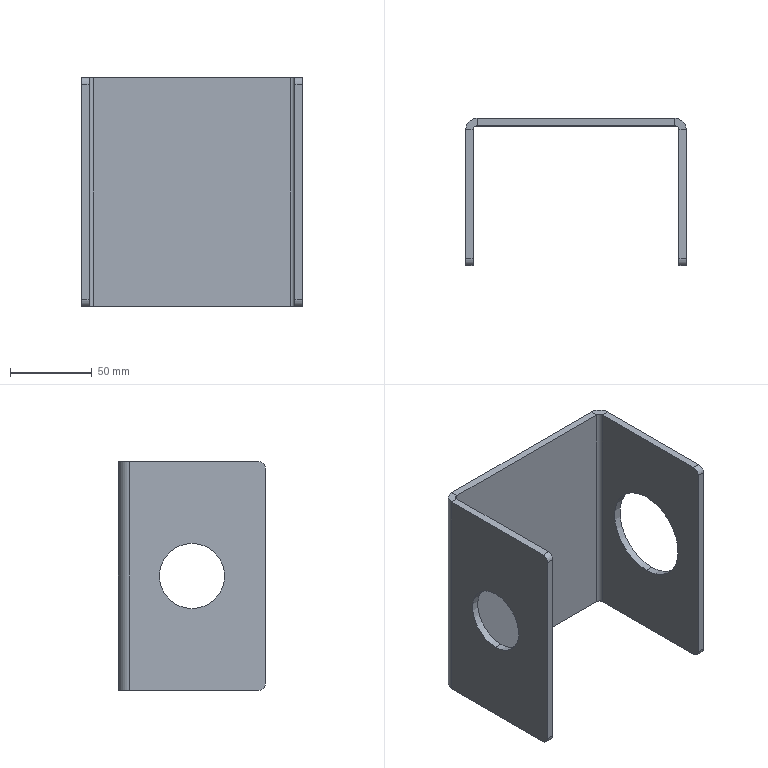Part | SolidWorks | features Cut 2, Fillet 1, FlatPattern 1, SMBaseFlange 1, SheetMetal 1, UnFold 1 | 1 solid | 30 faces | box 135 x 90 x 140 mm | volume 173803 mm3 | plane 18 | cylinder 12 | commonest cylinder face diameters 8 x4 5 x2 14 x2 40 x2 55 x2
STEP:
#1=CARTESIAN_POINT('',(63.,-45.,27.5));
#2=VERTEX_POINT('',#1);
#3=CARTESIAN_POINT('',(63.,-45.,-27.5));
#4=VERTEX_POINT('',#3);
#5=CARTESIAN_POINT('',(63.,-45.,0.));
#6=DIRECTION('',(1.,0.,0.));
#7=DIRECTION('',(0.,0.,-1.));
#8=AXIS2_PLACEMENT_3D('',#5,#6,#7);
#9=CIRCLE('',#8,27.5);
#10=EDGE_CURVE('',#2,#4,#9,.T.);
#11=ORIENTED_EDGE('',*,*,#10,.F.);
#12=CARTESIAN_POINT('',(67.5,-45.,27.5));
#13=VERTEX_POINT('',#12);
#14=CARTESIAN_POINT('',(57.5,-45.,27.5));
#15=DIRECTION('',(1.,0.,0.));
#16=VECTOR('',#15,1000.);
#17=LINE('',#14,#16);
#18=EDGE_CURVE('',#2,#13,#17,.T.);
#19=ORIENTED_EDGE('',*,*,#18,.T.);
#20=CARTESIAN_POINT('',(67.5,-45.,-27.5));
#21=VERTEX_POINT('',#20);
#22=CARTESIAN_POINT('',(67.5,-45.,0.));
#23=DIRECTION('',(1.,0.,0.));
#24=DIRECTION('',(0.,0.,-1.));
#25=AXIS2_PLACEMENT_3D('',#22,#23,#24);
#26=CIRCLE('',#25,27.5);
#27=EDGE_CURVE('',#13,#21,#26,.T.);
#28=ORIENTED_EDGE('',*,*,#27,.T.);
#29=CARTESIAN_POINT('',(57.5,-45.,-27.5));
#30=DIRECTION('',(1.,0.,0.));
#31=VECTOR('',#30,1000.);
#32=LINE('',#29,#31);
#33=EDGE_CURVE('',#4,#21,#32,.T.);
#34=ORIENTED_EDGE('',*,*,#33,.F.);
#35=EDGE_LOOP('',(#11,#19,#28,#34));
#36=FACE_OUTER_BOUND('',#35,.T.);
#37=CARTESIAN_POINT('',(57.5,-45.,0.));
#38=DIRECTION('',(1.,0.,0.));
#39=DIRECTION('',(0.,0.,-1.));
#40=AXIS2_PLACEMENT_3D('',#37,#38,#39);
#41=CYLINDRICAL_SURFACE('',#40,27.5);
#42=ADVANCED_FACE('',(#36),#41,.F.);
#43=CARTESIAN_POINT('',(-63.,-45.,-20.));
#44=VERTEX_POINT('',#43);
#45=CARTESIAN_POINT('',(-63.,-45.,20.));
#46=VERTEX_POINT('',#45);
#47=CARTESIAN_POINT('',(-63.,-45.,0.));
#48=DIRECTION('',(-1.,0.,0.));
#49=DIRECTION('',(0.,0.,1.));
#50=AXIS2_PLACEMENT_3D('',#47,#48,#49);
#51=CIRCLE('',#50,20.);
#52=EDGE_CURVE('',#44,#46,#51,.T.);
#53=ORIENTED_EDGE('',*,*,#52,.F.);
#54=CARTESIAN_POINT('',(-67.5,-45.,-20.));
#55=VERTEX_POINT('',#54);
#56=CARTESIAN_POINT('',(-57.5,-45.,-20.));
#57=DIRECTION('',(-1.,0.,0.));
#58=VECTOR('',#57,1000.);
#59=LINE('',#56,#58);
#60=EDGE_CURVE('',#44,#55,#59,.T.);
#61=ORIENTED_EDGE('',*,*,#60,.T.);
#62=CARTESIAN_POINT('',(-67.5,-45.,20.));
#63=VERTEX_POINT('',#62);
#64=CARTESIAN_POINT('',(-67.5,-45.,0.));
#65=DIRECTION('',(-1.,0.,0.));
#66=DIRECTION('',(0.,0.,1.));
#67=AXIS2_PLACEMENT_3D('',#64,#65,#66);
#68=CIRCLE('',#67,20.);
#69=EDGE_CURVE('',#55,#63,#68,.T.);
#70=ORIENTED_EDGE('',*,*,#69,.T.);
#71=CARTESIAN_POINT('',(-57.5,-45.,20.));
#72=DIRECTION('',(-1.,0.,0.));
#73=VECTOR('',#72,1000.);
#74=LINE('',#71,#73);
#75=EDGE_CURVE('',#46,#63,#74,.T.);
#76=ORIENTED_EDGE('',*,*,#75,.F.);
#77=EDGE_LOOP('',(#53,#61,#70,#76));
#78=FACE_OUTER_BOUND('',#77,.T.);
#79=CARTESIAN_POINT('',(-57.5,-45.,0.));
#80=DIRECTION('',(-1.,0.,0.));
#81=DIRECTION('',(0.,0.,1.));
#82=AXIS2_PLACEMENT_3D('',#79,#80,#81);
#83=CYLINDRICAL_SURFACE('',#82,20.);
#84=ADVANCED_FACE('',(#78),#83,.F.);
#85=CARTESIAN_POINT('',(-60.5,0.,70.));
#86=VERTEX_POINT('',#85);
#87=CARTESIAN_POINT('',(-60.5,-4.5,70.));
#88=VERTEX_POINT('',#87);
#89=CARTESIAN_POINT('',(-60.5,0.,70.));
#90=DIRECTION('',(0.,-1.,0.));
#91=VECTOR('',#90,1000.);
#92=LINE('',#89,#91);
#93=EDGE_CURVE('',#86,#88,#92,.T.);
#94=ORIENTED_EDGE('',*,*,#93,.F.);
#95=CARTESIAN_POINT('',(-67.5,-7.,70.));
#96=VERTEX_POINT('',#95);
#97=CARTESIAN_POINT('',(-60.5,-7.,70.));
#98=DIRECTION('',(0.,0.,-1.));
#99=DIRECTION('',(1.,0.,0.));
#100=AXIS2_PLACEMENT_3D('',#97,#98,#99);
#101=CIRCLE('',#100,7.);
#102=EDGE_CURVE('',#96,#86,#101,.T.);
#103=ORIENTED_EDGE('',*,*,#102,.F.);
#104=CARTESIAN_POINT('',(-63.,-7.,70.));
#105=VERTEX_POINT('',#104);
#106=CARTESIAN_POINT('',(-63.,-7.,70.));
#107=DIRECTION('',(-1.,0.,0.));
#108=VECTOR('',#107,1000.);
#109=LINE('',#106,#108);
#110=EDGE_CURVE('',#105,#96,#109,.T.);
#111=ORIENTED_EDGE('',*,*,#110,.F.);
#112=CARTESIAN_POINT('',(-60.5,-7.,70.));
#113=DIRECTION('',(0.,0.,-1.));
#114=DIRECTION('',(1.,0.,0.));
#115=AXIS2_PLACEMENT_3D('',#112,#113,#114);
#116=CIRCLE('',#115,2.5);
#117=EDGE_CURVE('',#105,#88,#116,.T.);
#118=ORIENTED_EDGE('',*,*,#117,.T.);
#119=EDGE_LOOP('',(#94,#103,#111,#118));
#120=FACE_OUTER_BOUND('',#119,.T.);
#121=CARTESIAN_POINT('',(-60.5,0.,70.));
#122=DIRECTION('',(0.,0.,1.));
#123=DIRECTION('',(1.,0.,0.));
#124=AXIS2_PLACEMENT_3D('',#121,#122,#123);
#125=PLANE('',#124);
#126=ADVANCED_FACE('',(#120),#125,.T.);
#127=CARTESIAN_POINT('',(60.5,0.,70.));
#128=VERTEX_POINT('',#127);
#129=CARTESIAN_POINT('',(-67.5,0.,70.));
#130=DIRECTION('',(1.,0.,0.));
#131=VECTOR('',#130,1000.);
#132=LINE('',#129,#131);
#133=EDGE_CURVE('',#86,#128,#132,.T.);
#134=ORIENTED_EDGE('',*,*,#133,.F.);
#135=ORIENTED_EDGE('',*,*,#93,.T.);
#136=CARTESIAN_POINT('',(60.5,-4.5,70.));
#137=VERTEX_POINT('',#136);
#138=CARTESIAN_POINT('',(-67.5,-4.5,70.));
#139=DIRECTION('',(1.,0.,0.));
#140=VECTOR('',#139,1000.);
#141=LINE('',#138,#140);
#142=EDGE_CURVE('',#88,#137,#141,.T.);
#143=ORIENTED_EDGE('',*,*,#142,.T.);
#144=CARTESIAN_POINT('',(60.5,-4.5,70.));
#145=DIRECTION('',(0.,1.,0.));
#146=VECTOR('',#145,1000.);
#147=LINE('',#144,#146);
#148=EDGE_CURVE('',#137,#128,#147,.T.);
#149=ORIENTED_EDGE('',*,*,#148,.T.);
#150=EDGE_LOOP('',(#134,#135,#143,#149));
#151=FACE_OUTER_BOUND('',#150,.T.);
#152=CARTESIAN_POINT('',(-63.,-7.,70.));
#153=DIRECTION('',(0.,0.,1.));
#154=DIRECTION('',(1.,0.,0.));
#155=AXIS2_PLACEMENT_3D('',#152,#153,#154);
#156=PLANE('',#155);
#157=ADVANCED_FACE('',(#151),#156,.T.);
#158=CARTESIAN_POINT('',(-67.5,-7.,-70.));
#159=VERTEX_POINT('',#158);
#160=CARTESIAN_POINT('',(-63.,-7.,-70.));
#161=VERTEX_POINT('',#160);
#162=CARTESIAN_POINT('',(-67.5,-7.,-70.));
#163=DIRECTION('',(1.,0.,0.));
#164=VECTOR('',#163,1000.);
#165=LINE('',#162,#164);
#166=EDGE_CURVE('',#159,#161,#165,.T.);
#167=ORIENTED_EDGE('',*,*,#166,.F.);
#168=CARTESIAN_POINT('',(-60.5,0.,-70.));
#169=VERTEX_POINT('',#168);
#170=CARTESIAN_POINT('',(-60.5,-7.,-70.));
#171=DIRECTION('',(0.,0.,-1.));
#172=DIRECTION('',(1.,0.,0.));
#173=AXIS2_PLACEMENT_3D('',#170,#171,#172);
#174=CIRCLE('',#173,7.);
#175=EDGE_CURVE('',#159,#169,#174,.T.);
#176=ORIENTED_EDGE('',*,*,#175,.T.);
#177=CARTESIAN_POINT('',(-60.5,-4.5,-70.));
#178=VERTEX_POINT('',#177);
#179=CARTESIAN_POINT('',(-60.5,-4.5,-70.));
#180=DIRECTION('',(0.,1.,0.));
#181=VECTOR('',#180,1000.);
#182=LINE('',#179,#181);
#183=EDGE_CURVE('',#178,#169,#182,.T.);
#184=ORIENTED_EDGE('',*,*,#183,.F.);
#185=CARTESIAN_POINT('',(-60.5,-7.,-70.));
#186=DIRECTION('',(0.,0.,-1.));
#187=DIRECTION('',(1.,0.,0.));
#188=AXIS2_PLACEMENT_3D('',#185,#186,#187);
#189=CIRCLE('',#188,2.5);
#190=EDGE_CURVE('',#161,#178,#189,.T.);
#191=ORIENTED_EDGE('',*,*,#190,.F.);
#192=EDGE_LOOP('',(#167,#176,#184,#191));
#193=FACE_OUTER_BOUND('',#192,.T.);
#194=CARTESIAN_POINT('',(-67.5,-7.,-70.));
#195=DIRECTION('',(0.,0.,-1.));
#196=DIRECTION('',(-1.,0.,0.));
#197=AXIS2_PLACEMENT_3D('',#194,#195,#196);
#198=PLANE('',#197);
#199=ADVANCED_FACE('',(#193),#198,.T.);
#200=CARTESIAN_POINT('',(-63.,-86.,-70.));
#201=VERTEX_POINT('',#200);
#202=CARTESIAN_POINT('',(-63.,-90.,-70.));
#203=DIRECTION('',(0.,1.,0.));
#204=VECTOR('',#203,1000.);
#205=LINE('',#202,#204);
#206=EDGE_CURVE('',#201,#161,#205,.T.);
#207=ORIENTED_EDGE('',*,*,#206,.F.);
#208=CARTESIAN_POINT('',(-67.5,-86.,-70.));
#209=VERTEX_POINT('',#208);
#210=CARTESIAN_POINT('',(-60.5,-86.,-70.));
#211=DIRECTION('',(-1.,0.,0.));
#212=VECTOR('',#211,1000.);
#213=LINE('',#210,#212);
#214=EDGE_CURVE('',#201,#209,#213,.T.);
#215=ORIENTED_EDGE('',*,*,#214,.T.);
#216=CARTESIAN_POINT('',(-67.5,-90.,-70.));
#217=DIRECTION('',(0.,1.,0.));
#218=VECTOR('',#217,1000.);
#219=LINE('',#216,#218);
#220=EDGE_CURVE('',#209,#159,#219,.T.);
#221=ORIENTED_EDGE('',*,*,#220,.T.);
#222=ORIENTED_EDGE('',*,*,#166,.T.);
#223=EDGE_LOOP('',(#207,#215,#221,#222));
#224=FACE_OUTER_BOUND('',#223,.T.);
#225=CARTESIAN_POINT('',(-60.5,-4.5,-70.));
#226=DIRECTION('',(0.,0.,-1.));
#227=DIRECTION('',(-1.,0.,0.));
#228=AXIS2_PLACEMENT_3D('',#225,#226,#227);
#229=PLANE('',#228);
#230=ADVANCED_FACE('',(#224),#229,.T.);
#231=CARTESIAN_POINT('',(67.5,-7.,70.));
#232=VERTEX_POINT('',#231);
#233=CARTESIAN_POINT('',(63.,-7.,70.));
#234=VERTEX_POINT('',#233);
#235=CARTESIAN_POINT('',(67.5,-7.,70.));
#236=DIRECTION('',(-1.,0.,0.));
#237=VECTOR('',#236,1000.);
#238=LINE('',#235,#237);
#239=EDGE_CURVE('',#232,#234,#238,.T.);
#240=ORIENTED_EDGE('',*,*,#239,.F.);
#241=CARTESIAN_POINT('',(60.5,-7.,70.));
#242=DIRECTION('',(0.,0.,-1.));
#243=DIRECTION('',(1.,0.,0.));
#244=AXIS2_PLACEMENT_3D('',#241,#242,#243);
#245=CIRCLE('',#244,7.);
#246=EDGE_CURVE('',#128,#232,#245,.T.);
#247=ORIENTED_EDGE('',*,*,#246,.F.);
#248=ORIENTED_EDGE('',*,*,#148,.F.);
#249=CARTESIAN_POINT('',(60.5,-7.,70.));
#250=DIRECTION('',(0.,0.,-1.));
#251=DIRECTION('',(1.,0.,0.));
#252=AXIS2_PLACEMENT_3D('',#249,#250,#251);
#253=CIRCLE('',#252,2.5);
#254=EDGE_CURVE('',#137,#234,#253,.T.);
#255=ORIENTED_EDGE('',*,*,#254,.T.);
#256=EDGE_LOOP('',(#240,#247,#248,#255));
#257=FACE_OUTER_BOUND('',#256,.T.);
#258=CARTESIAN_POINT('',(67.5,-7.,70.));
#259=DIRECTION('',(0.,0.,1.));
#260=DIRECTION('',(1.,0.,0.));
#261=AXIS2_PLACEMENT_3D('',#258,#259,#260);
#262=PLANE('',#261);
#263=ADVANCED_FACE('',(#257),#262,.T.);
#264=CARTESIAN_POINT('',(63.,-86.,70.));
#265=VERTEX_POINT('',#264);
#266=CARTESIAN_POINT('',(63.,0.,70.));
#267=DIRECTION('',(0.,-1.,0.));
#268=VECTOR('',#267,1000.);
#269=LINE('',#266,#268);
#270=EDGE_CURVE('',#234,#265,#269,.T.);
#271=ORIENTED_EDGE('',*,*,#270,.T.);
#272=CARTESIAN_POINT('',(67.5,-86.,70.));
#273=VERTEX_POINT('',#272);
#274=CARTESIAN_POINT('',(60.5,-86.,70.));
#275=DIRECTION('',(1.,0.,0.));
#276=VECTOR('',#275,1000.);
#277=LINE('',#274,#276);
#278=EDGE_CURVE('',#265,#273,#277,.T.);
#279=ORIENTED_EDGE('',*,*,#278,.T.);
#280=CARTESIAN_POINT('',(67.5,0.,70.));
#281=DIRECTION('',(0.,-1.,0.));
#282=VECTOR('',#281,1000.);
#283=LINE('',#280,#282);
#284=EDGE_CURVE('',#232,#273,#283,.T.);
#285=ORIENTED_EDGE('',*,*,#284,.F.);
#286=ORIENTED_EDGE('',*,*,#239,.T.);
#287=EDGE_LOOP('',(#271,#279,#285,#286));
#288=FACE_OUTER_BOUND('',#287,.T.);
#289=CARTESIAN_POINT('',(60.5,-4.5,70.));
#290=DIRECTION('',(0.,0.,1.));
#291=DIRECTION('',(1.,0.,0.));
#292=AXIS2_PLACEMENT_3D('',#289,#290,#291);
#293=PLANE('',#292);
#294=ADVANCED_FACE('',(#288),#293,.T.);
#295=CARTESIAN_POINT('',(60.5,0.,-70.));
#296=VERTEX_POINT('',#295);
#297=CARTESIAN_POINT('',(60.5,-4.5,-70.));
#298=VERTEX_POINT('',#297);
#299=CARTESIAN_POINT('',(60.5,0.,-70.));
#300=DIRECTION('',(0.,-1.,0.));
#301=VECTOR('',#300,1000.);
#302=LINE('',#299,#301);
#303=EDGE_CURVE('',#296,#298,#302,.T.);
#304=ORIENTED_EDGE('',*,*,#303,.F.);
#305=CARTESIAN_POINT('',(67.5,-7.,-70.));
#306=VERTEX_POINT('',#305);
#307=CARTESIAN_POINT('',(60.5,-7.,-70.));
#308=DIRECTION('',(0.,0.,-1.));
#309=DIRECTION('',(1.,0.,0.));
#310=AXIS2_PLACEMENT_3D('',#307,#308,#309);
#311=CIRCLE('',#310,7.);
#312=EDGE_CURVE('',#296,#306,#311,.T.);
#313=ORIENTED_EDGE('',*,*,#312,.T.);
#314=CARTESIAN_POINT('',(63.,-7.,-70.));
#315=VERTEX_POINT('',#314);
#316=CARTESIAN_POINT('',(63.,-7.,-70.));
#317=DIRECTION('',(1.,0.,0.));
#318=VECTOR('',#317,1000.);
#319=LINE('',#316,#318);
#320=EDGE_CURVE('',#315,#306,#319,.T.);
#321=ORIENTED_EDGE('',*,*,#320,.F.);
#322=CARTESIAN_POINT('',(60.5,-7.,-70.));
#323=DIRECTION('',(0.,0.,-1.));
#324=DIRECTION('',(1.,0.,0.));
#325=AXIS2_PLACEMENT_3D('',#322,#323,#324);
#326=CIRCLE('',#325,2.5);
#327=EDGE_CURVE('',#298,#315,#326,.T.);
#328=ORIENTED_EDGE('',*,*,#327,.F.);
#329=EDGE_LOOP('',(#304,#313,#321,#328));
#330=FACE_OUTER_BOUND('',#329,.T.);
#331=CARTESIAN_POINT('',(60.5,0.,-70.));
#332=DIRECTION('',(0.,0.,-1.));
#333=DIRECTION('',(-1.,0.,0.));
#334=AXIS2_PLACEMENT_3D('',#331,#332,#333);
#335=PLANE('',#334);
#336=ADVANCED_FACE('',(#330),#335,.T.);
#337=CARTESIAN_POINT('',(-67.5,0.,-70.));
#338=DIRECTION('',(1.,0.,0.));
#339=VECTOR('',#338,1000.);
#340=LINE('',#337,#339);
#341=EDGE_CURVE('',#169,#296,#340,.T.);
#342=ORIENTED_EDGE('',*,*,#341,.T.);
#343=ORIENTED_EDGE('',*,*,#303,.T.);
#344=CARTESIAN_POINT('',(-67.5,-4.5,-70.));
#345=DIRECTION('',(1.,0.,0.));
#346=VECTOR('',#345,1000.);
#347=LINE('',#344,#346);
#348=EDGE_CURVE('',#178,#298,#347,.T.);
#349=ORIENTED_EDGE('',*,*,#348,.F.);
#350=ORIENTED_EDGE('',*,*,#183,.T.);
#351=EDGE_LOOP('',(#342,#343,#349,#350));
#352=FACE_OUTER_BOUND('',#351,.T.);
#353=CARTESIAN_POINT('',(63.,-7.,-70.));
#354=DIRECTION('',(0.,0.,-1.));
#355=DIRECTION('',(-1.,0.,0.));
#356=AXIS2_PLACEMENT_3D('',#353,#354,#355);
#357=PLANE('',#356);
#358=ADVANCED_FACE('',(#352),#357,.T.);
#359=CARTESIAN_POINT('',(63.,-45.,0.));
#360=DIRECTION('',(1.,0.,0.));
#361=DIRECTION('',(0.,0.,-1.));
#362=AXIS2_PLACEMENT_3D('',#359,#360,#361);
#363=CIRCLE('',#362,27.5);
#364=EDGE_CURVE('',#4,#2,#363,.T.);
#365=ORIENTED_EDGE('',*,*,#364,.T.);
#366=ORIENTED_EDGE('',*,*,#10,.T.);
#367=EDGE_LOOP('',(#365,#366));
#368=FACE_BOUND('',#367,.T.);
#369=CARTESIAN_POINT('',(63.,-86.,-70.));
#370=VERTEX_POINT('',#369);
#371=CARTESIAN_POINT('',(63.,0.,-70.));
#372=DIRECTION('',(0.,-1.,0.));
#373=VECTOR('',#372,1000.);
#374=LINE('',#371,#373);
#375=EDGE_CURVE('',#315,#370,#374,.T.);
#376=ORIENTED_EDGE('',*,*,#375,.T.);
#377=CARTESIAN_POINT('',(63.,-90.,-66.));
#378=VERTEX_POINT('',#377);
#379=CARTESIAN_POINT('',(63.,-86.,-66.));
#380=DIRECTION('',(-1.,0.,0.));
#381=DIRECTION('',(0.,0.,-1.));
#382=AXIS2_PLACEMENT_3D('',#379,#380,#381);
#383=CIRCLE('',#382,4.);
#384=EDGE_CURVE('',#370,#378,#383,.T.);
#385=ORIENTED_EDGE('',*,*,#384,.T.);
#386=CARTESIAN_POINT('',(63.,-90.,66.));
#387=VERTEX_POINT('',#386);
#388=CARTESIAN_POINT('',(63.,-90.,70.));
#389=DIRECTION('',(0.,0.,-1.));
#390=VECTOR('',#389,1000.);
#391=LINE('',#388,#390);
#392=EDGE_CURVE('',#387,#378,#391,.T.);
#393=ORIENTED_EDGE('',*,*,#392,.F.);
#394=CARTESIAN_POINT('',(63.,-86.,66.));
#395=DIRECTION('',(-1.,0.,0.));
#396=DIRECTION('',(0.,0.,-1.));
#397=AXIS2_PLACEMENT_3D('',#394,#395,#396);
#398=CIRCLE('',#397,4.);
#399=EDGE_CURVE('',#387,#265,#398,.T.);
#400=ORIENTED_EDGE('',*,*,#399,.T.);
#401=ORIENTED_EDGE('',*,*,#270,.F.);
#402=CARTESIAN_POINT('',(63.,-7.,70.));
#403=DIRECTION('',(0.,0.,-1.));
#404=VECTOR('',#403,1000.);
#405=LINE('',#402,#404);
#406=EDGE_CURVE('',#234,#315,#405,.T.);
#407=ORIENTED_EDGE('',*,*,#406,.T.);
#408=EDGE_LOOP('',(#376,#385,#393,#400,#401,#407));
#409=FACE_OUTER_BOUND('',#408,.T.);
#410=CARTESIAN_POINT('',(63.,0.,70.));
#411=DIRECTION('',(1.,0.,0.));
#412=DIRECTION('',(0.,0.,-1.));
#413=AXIS2_PLACEMENT_3D('',#410,#411,#412);
#414=PLANE('',#413);
#415=ADVANCED_FACE('',(#368,#409),#414,.F.);
#416=ORIENTED_EDGE('',*,*,#392,.T.);
#417=CARTESIAN_POINT('',(67.5,-90.,-66.));
#418=VERTEX_POINT('',#417);
#419=CARTESIAN_POINT('',(67.5,-90.,-66.));
#420=DIRECTION('',(1.,0.,0.));
#421=VECTOR('',#420,1000.);
#422=LINE('',#419,#421);
#423=EDGE_CURVE('',#378,#418,#422,.T.);
#424=ORIENTED_EDGE('',*,*,#423,.T.);
#425=CARTESIAN_POINT('',(67.5,-90.,66.));
#426=VERTEX_POINT('',#425);
#427=CARTESIAN_POINT('',(67.5,-90.,70.));
#428=DIRECTION('',(0.,0.,-1.));
#429=VECTOR('',#428,1000.);
#430=LINE('',#427,#429);
#431=EDGE_CURVE('',#426,#418,#430,.T.);
#432=ORIENTED_EDGE('',*,*,#431,.F.);
#433=CARTESIAN_POINT('',(67.5,-90.,66.));
#434=DIRECTION('',(-1.,0.,0.));
#435=VECTOR('',#434,1000.);
#436=LINE('',#433,#435);
#437=EDGE_CURVE('',#426,#387,#436,.T.);
#438=ORIENTED_EDGE('',*,*,#437,.T.);
#439=EDGE_LOOP('',(#416,#424,#432,#438));
#440=FACE_OUTER_BOUND('',#439,.T.);
#441=CARTESIAN_POINT('',(67.5,-90.,70.));
#442=DIRECTION('',(0.,-1.,0.));
#443=DIRECTION('',(0.,0.,-1.));
#444=AXIS2_PLACEMENT_3D('',#441,#442,#443);
#445=PLANE('',#444);
#446=ADVANCED_FACE('',(#440),#445,.T.);
#447=CARTESIAN_POINT('',(67.5,-45.,0.));
#448=DIRECTION('',(1.,0.,0.));
#449=DIRECTION('',(0.,0.,-1.));
#450=AXIS2_PLACEMENT_3D('',#447,#448,#449);
#451=CIRCLE('',#450,27.5);
#452=EDGE_CURVE('',#21,#13,#451,.T.);
#453=ORIENTED_EDGE('',*,*,#452,.F.);
#454=ORIENTED_EDGE('',*,*,#27,.F.);
#455=EDGE_LOOP('',(#453,#454));
#456=FACE_BOUND('',#455,.T.);
#457=ORIENTED_EDGE('',*,*,#431,.T.);
#458=CARTESIAN_POINT('',(67.5,-86.,-70.));
#459=VERTEX_POINT('',#458);
#460=CARTESIAN_POINT('',(67.5,-86.,-66.));
#461=DIRECTION('',(1.,0.,0.));
#462=DIRECTION('',(0.,0.,-1.));
#463=AXIS2_PLACEMENT_3D('',#460,#461,#462);
#464=CIRCLE('',#463,4.);
#465=EDGE_CURVE('',#418,#459,#464,.T.);
#466=ORIENTED_EDGE('',*,*,#465,.T.);
#467=CARTESIAN_POINT('',(67.5,0.,-70.));
#468=DIRECTION('',(0.,-1.,0.));
#469=VECTOR('',#468,1000.);
#470=LINE('',#467,#469);
#471=EDGE_CURVE('',#306,#459,#470,.T.);
#472=ORIENTED_EDGE('',*,*,#471,.F.);
#473=CARTESIAN_POINT('',(67.5,-7.,70.));
#474=DIRECTION('',(0.,0.,-1.));
#475=VECTOR('',#474,1000.);
#476=LINE('',#473,#475);
#477=EDGE_CURVE('',#232,#306,#476,.T.);
#478=ORIENTED_EDGE('',*,*,#477,.F.);
#479=ORIENTED_EDGE('',*,*,#284,.T.);
#480=CARTESIAN_POINT('',(67.5,-86.,66.));
#481=DIRECTION('',(1.,0.,0.));
#482=DIRECTION('',(0.,0.,-1.));
#483=AXIS2_PLACEMENT_3D('',#480,#481,#482);
#484=CIRCLE('',#483,4.);
#485=EDGE_CURVE('',#273,#426,#484,.T.);
#486=ORIENTED_EDGE('',*,*,#485,.T.);
#487=EDGE_LOOP('',(#457,#466,#472,#478,#479,#486));
#488=FACE_OUTER_BOUND('',#487,.T.);
#489=CARTESIAN_POINT('',(67.5,0.,70.));
#490=DIRECTION('',(1.,0.,0.));
#491=DIRECTION('',(0.,0.,-1.));
#492=AXIS2_PLACEMENT_3D('',#489,#490,#491);
#493=PLANE('',#492);
#494=ADVANCED_FACE('',(#456,#488),#493,.T.);
#495=ORIENTED_EDGE('',*,*,#312,.F.);
#496=CARTESIAN_POINT('',(60.5,0.,70.));
#497=DIRECTION('',(0.,0.,-1.));
#498=VECTOR('',#497,1000.);
#499=LINE('',#496,#498);
#500=EDGE_CURVE('',#128,#296,#499,.T.);
#501=ORIENTED_EDGE('',*,*,#500,.F.);
#502=ORIENTED_EDGE('',*,*,#246,.T.);
#503=ORIENTED_EDGE('',*,*,#477,.T.);
#504=EDGE_LOOP('',(#495,#501,#502,#503));
#505=FACE_OUTER_BOUND('',#504,.T.);
#506=CARTESIAN_POINT('',(60.5,-7.,70.));
#507=DIRECTION('',(0.,0.,-1.));
#508=DIRECTION('',(-1.,0.,0.));
#509=AXIS2_PLACEMENT_3D('',#506,#507,#508);
#510=CYLINDRICAL_SURFACE('',#509,7.);
#511=ADVANCED_FACE('',(#505),#510,.T.);
#512=ORIENTED_EDGE('',*,*,#341,.F.);
#513=CARTESIAN_POINT('',(-60.5,0.,70.));
#514=DIRECTION('',(0.,0.,-1.));
#515=VECTOR('',#514,1000.);
#516=LINE('',#513,#515);
#517=EDGE_CURVE('',#86,#169,#516,.T.);
#518=ORIENTED_EDGE('',*,*,#517,.F.);
#519=ORIENTED_EDGE('',*,*,#133,.T.);
#520=ORIENTED_EDGE('',*,*,#500,.T.);
#521=EDGE_LOOP('',(#512,#518,#519,#520));
#522=FACE_OUTER_BOUND('',#521,.T.);
#523=CARTESIAN_POINT('',(-67.5,0.,70.));
#524=DIRECTION('',(0.,1.,0.));
#525=DIRECTION('',(0.,0.,1.));
#526=AXIS2_PLACEMENT_3D('',#523,#524,#525);
#527=PLANE('',#526);
#528=ADVANCED_FACE('',(#522),#527,.T.);
#529=ORIENTED_EDGE('',*,*,#175,.F.);
#530=CARTESIAN_POINT('',(-67.5,-7.,70.));
#531=DIRECTION('',(0.,0.,-1.));
#532=VECTOR('',#531,1000.);
#533=LINE('',#530,#532);
#534=EDGE_CURVE('',#96,#159,#533,.T.);
#535=ORIENTED_EDGE('',*,*,#534,.F.);
#536=ORIENTED_EDGE('',*,*,#102,.T.);
#537=ORIENTED_EDGE('',*,*,#517,.T.);
#538=EDGE_LOOP('',(#529,#535,#536,#537));
#539=FACE_OUTER_BOUND('',#538,.T.);
#540=CARTESIAN_POINT('',(-60.5,-7.,70.));
#541=DIRECTION('',(0.,0.,-1.));
#542=DIRECTION('',(-1.,0.,0.));
#543=AXIS2_PLACEMENT_3D('',#540,#541,#542);
#544=CYLINDRICAL_SURFACE('',#543,7.);
#545=ADVANCED_FACE('',(#539),#544,.T.);
#546=CARTESIAN_POINT('',(-67.5,-45.,0.));
#547=DIRECTION('',(-1.,0.,0.));
#548=DIRECTION('',(0.,0.,1.));
#549=AXIS2_PLACEMENT_3D('',#546,#547,#548);
#550=CIRCLE('',#549,20.);
#551=EDGE_CURVE('',#63,#55,#550,.T.);
#552=ORIENTED_EDGE('',*,*,#551,.F.);
#553=ORIENTED_EDGE('',*,*,#69,.F.);
#554=EDGE_LOOP('',(#552,#553));
#555=FACE_BOUND('',#554,.T.);
#556=ORIENTED_EDGE('',*,*,#220,.F.);
#557=CARTESIAN_POINT('',(-67.5,-90.,-66.));
#558=VERTEX_POINT('',#557);
#559=CARTESIAN_POINT('',(-67.5,-86.,-66.));
#560=DIRECTION('',(-1.,0.,0.));
#561=DIRECTION('',(0.,0.,1.));
#562=AXIS2_PLACEMENT_3D('',#559,#560,#561);
#563=CIRCLE('',#562,4.);
#564=EDGE_CURVE('',#209,#558,#563,.T.);
#565=ORIENTED_EDGE('',*,*,#564,.T.);
#566=CARTESIAN_POINT('',(-67.5,-90.,66.));
#567=VERTEX_POINT('',#566);
#568=CARTESIAN_POINT('',(-67.5,-90.,70.));
#569=DIRECTION('',(0.,0.,-1.));
#570=VECTOR('',#569,1000.);
#571=LINE('',#568,#570);
#572=EDGE_CURVE('',#567,#558,#571,.T.);
#573=ORIENTED_EDGE('',*,*,#572,.F.);
#574=CARTESIAN_POINT('',(-67.5,-86.,70.));
#575=VERTEX_POINT('',#574);
#576=CARTESIAN_POINT('',(-67.5,-86.,66.));
#577=DIRECTION('',(-1.,0.,0.));
#578=DIRECTION('',(0.,0.,1.));
#579=AXIS2_PLACEMENT_3D('',#576,#577,#578);
#580=CIRCLE('',#579,4.);
#581=EDGE_CURVE('',#567,#575,#580,.T.);
#582=ORIENTED_EDGE('',*,*,#581,.T.);
#583=CARTESIAN_POINT('',(-67.5,-90.,70.));
#584=DIRECTION('',(0.,1.,0.));
#585=VECTOR('',#584,1000.);
#586=LINE('',#583,#585);
#587=EDGE_CURVE('',#575,#96,#586,.T.);
#588=ORIENTED_EDGE('',*,*,#587,.T.);
#589=ORIENTED_EDGE('',*,*,#534,.T.);
#590=EDGE_LOOP('',(#556,#565,#573,#582,#588,#589));
#591=FACE_OUTER_BOUND('',#590,.T.);
#592=CARTESIAN_POINT('',(-67.5,-90.,70.));
#593=DIRECTION('',(-1.,0.,0.));
#594=DIRECTION('',(0.,0.,1.));
#595=AXIS2_PLACEMENT_3D('',#592,#593,#594);
#596=PLANE('',#595);
#597=ADVANCED_FACE('',(#555,#591),#596,.T.);
#598=ORIENTED_EDGE('',*,*,#572,.T.);
#599=CARTESIAN_POINT('',(-63.,-90.,-66.));
#600=VERTEX_POINT('',#599);
#601=CARTESIAN_POINT('',(-63.,-90.,-66.));
#602=DIRECTION('',(1.,0.,0.));
#603=VECTOR('',#602,1000.);
#604=LINE('',#601,#603);
#605=EDGE_CURVE('',#558,#600,#604,.T.);
#606=ORIENTED_EDGE('',*,*,#605,.T.);
#607=CARTESIAN_POINT('',(-63.,-90.,66.));
#608=VERTEX_POINT('',#607);
#609=CARTESIAN_POINT('',(-63.,-90.,70.));
#610=DIRECTION('',(0.,0.,-1.));
#611=VECTOR('',#610,1000.);
#612=LINE('',#609,#611);
#613=EDGE_CURVE('',#608,#600,#612,.T.);
#614=ORIENTED_EDGE('',*,*,#613,.F.);
#615=CARTESIAN_POINT('',(-63.,-90.,66.));
#616=DIRECTION('',(-1.,0.,0.));
#617=VECTOR('',#616,1000.);
#618=LINE('',#615,#617);
#619=EDGE_CURVE('',#608,#567,#618,.T.);
#620=ORIENTED_EDGE('',*,*,#619,.T.);
#621=EDGE_LOOP('',(#598,#606,#614,#620));
#622=FACE_OUTER_BOUND('',#621,.T.);
#623=CARTESIAN_POINT('',(-63.,-90.,70.));
#624=DIRECTION('',(0.,-1.,0.));
#625=DIRECTION('',(0.,0.,-1.));
#626=AXIS2_PLACEMENT_3D('',#623,#624,#625);
#627=PLANE('',#626);
#628=ADVANCED_FACE('',(#622),#627,.T.);
#629=CARTESIAN_POINT('',(-63.,-45.,0.));
#630=DIRECTION('',(-1.,0.,0.));
#631=DIRECTION('',(0.,0.,1.));
#632=AXIS2_PLACEMENT_3D('',#629,#630,#631);
#633=CIRCLE('',#632,20.);
#634=EDGE_CURVE('',#46,#44,#633,.T.);
#635=ORIENTED_EDGE('',*,*,#634,.T.);
#636=ORIENTED_EDGE('',*,*,#52,.T.);
#637=EDGE_LOOP('',(#635,#636));
#638=FACE_BOUND('',#637,.T.);
#639=ORIENTED_EDGE('',*,*,#613,.T.);
#640=CARTESIAN_POINT('',(-63.,-86.,-66.));
#641=DIRECTION('',(1.,0.,0.));
#642=DIRECTION('',(0.,0.,1.));
#643=AXIS2_PLACEMENT_3D('',#640,#641,#642);
#644=CIRCLE('',#643,4.);
#645=EDGE_CURVE('',#600,#201,#644,.T.);
#646=ORIENTED_EDGE('',*,*,#645,.T.);
#647=ORIENTED_EDGE('',*,*,#206,.T.);
#648=CARTESIAN_POINT('',(-63.,-7.,70.));
#649=DIRECTION('',(0.,0.,-1.));
#650=VECTOR('',#649,1000.);
#651=LINE('',#648,#650);
#652=EDGE_CURVE('',#105,#161,#651,.T.);
#653=ORIENTED_EDGE('',*,*,#652,.F.);
#654=CARTESIAN_POINT('',(-63.,-86.,70.));
#655=VERTEX_POINT('',#654);
#656=CARTESIAN_POINT('',(-63.,-90.,70.));
#657=DIRECTION('',(0.,1.,0.));
#658=VECTOR('',#657,1000.);
#659=LINE('',#656,#658);
#660=EDGE_CURVE('',#655,#105,#659,.T.);
#661=ORIENTED_EDGE('',*,*,#660,.F.);
#662=CARTESIAN_POINT('',(-63.,-86.,66.));
#663=DIRECTION('',(1.,0.,0.));
#664=DIRECTION('',(0.,0.,1.));
#665=AXIS2_PLACEMENT_3D('',#662,#663,#664);
#666=CIRCLE('',#665,4.);
#667=EDGE_CURVE('',#655,#608,#666,.T.);
#668=ORIENTED_EDGE('',*,*,#667,.T.);
#669=EDGE_LOOP('',(#639,#646,#647,#653,#661,#668));
#670=FACE_OUTER_BOUND('',#669,.T.);
#671=CARTESIAN_POINT('',(-63.,-90.,70.));
#672=DIRECTION('',(-1.,0.,0.));
#673=DIRECTION('',(0.,0.,1.));
#674=AXIS2_PLACEMENT_3D('',#671,#672,#673);
#675=PLANE('',#674);
#676=ADVANCED_FACE('',(#638,#670),#675,.F.);
#677=ORIENTED_EDGE('',*,*,#190,.T.);
#678=CARTESIAN_POINT('',(-60.5,-4.5,70.));
#679=DIRECTION('',(0.,0.,-1.));
#680=VECTOR('',#679,1000.);
#681=LINE('',#678,#680);
#682=EDGE_CURVE('',#88,#178,#681,.T.);
#683=ORIENTED_EDGE('',*,*,#682,.F.);
#684=ORIENTED_EDGE('',*,*,#117,.F.);
#685=ORIENTED_EDGE('',*,*,#652,.T.);
#686=EDGE_LOOP('',(#677,#683,#684,#685));
#687=FACE_OUTER_BOUND('',#686,.T.);
#688=CARTESIAN_POINT('',(-60.5,-7.,70.));
#689=DIRECTION('',(0.,0.,-1.));
#690=DIRECTION('',(-1.,0.,0.));
#691=AXIS2_PLACEMENT_3D('',#688,#689,#690);
#692=CYLINDRICAL_SURFACE('',#691,2.5);
#693=ADVANCED_FACE('',(#687),#692,.F.);
#694=ORIENTED_EDGE('',*,*,#348,.T.);
#695=CARTESIAN_POINT('',(60.5,-4.5,70.));
#696=DIRECTION('',(0.,0.,-1.));
#697=VECTOR('',#696,1000.);
#698=LINE('',#695,#697);
#699=EDGE_CURVE('',#137,#298,#698,.T.);
#700=ORIENTED_EDGE('',*,*,#699,.F.);
#701=ORIENTED_EDGE('',*,*,#142,.F.);
#702=ORIENTED_EDGE('',*,*,#682,.T.);
#703=EDGE_LOOP('',(#694,#700,#701,#702));
#704=FACE_OUTER_BOUND('',#703,.T.);
#705=CARTESIAN_POINT('',(-67.5,-4.5,70.));
#706=DIRECTION('',(0.,1.,0.));
#707=DIRECTION('',(0.,0.,1.));
#708=AXIS2_PLACEMENT_3D('',#705,#706,#707);
#709=PLANE('',#708);
#710=ADVANCED_FACE('',(#704),#709,.F.);
#711=ORIENTED_EDGE('',*,*,#327,.T.);
#712=ORIENTED_EDGE('',*,*,#406,.F.);
#713=ORIENTED_EDGE('',*,*,#254,.F.);
#714=ORIENTED_EDGE('',*,*,#699,.T.);
#715=EDGE_LOOP('',(#711,#712,#713,#714));
#716=FACE_OUTER_BOUND('',#715,.T.);
#717=CARTESIAN_POINT('',(60.5,-7.,70.));
#718=DIRECTION('',(0.,0.,-1.));
#719=DIRECTION('',(-1.,0.,0.));
#720=AXIS2_PLACEMENT_3D('',#717,#718,#719);
#721=CYLINDRICAL_SURFACE('',#720,2.5);
#722=ADVANCED_FACE('',(#716),#721,.F.);
#723=ORIENTED_EDGE('',*,*,#587,.F.);
#724=CARTESIAN_POINT('',(60.5,-86.,70.));
#725=DIRECTION('',(1.,0.,0.));
#726=VECTOR('',#725,1000.);
#727=LINE('',#724,#726);
#728=EDGE_CURVE('',#575,#655,#727,.T.);
#729=ORIENTED_EDGE('',*,*,#728,.T.);
#730=ORIENTED_EDGE('',*,*,#660,.T.);
#731=ORIENTED_EDGE('',*,*,#110,.T.);
#732=EDGE_LOOP('',(#723,#729,#730,#731));
#733=FACE_OUTER_BOUND('',#732,.T.);
#734=CARTESIAN_POINT('',(60.5,-7.,70.));
#735=DIRECTION('',(0.,0.,1.));
#736=DIRECTION('',(1.,0.,0.));
#737=AXIS2_PLACEMENT_3D('',#734,#735,#736);
#738=PLANE('',#737);
#739=ADVANCED_FACE('',(#733),#738,.T.);
#740=ORIENTED_EDGE('',*,*,#471,.T.);
#741=CARTESIAN_POINT('',(63.,-86.,-70.));
#742=DIRECTION('',(-1.,0.,0.));
#743=VECTOR('',#742,1000.);
#744=LINE('',#741,#743);
#745=EDGE_CURVE('',#459,#370,#744,.T.);
#746=ORIENTED_EDGE('',*,*,#745,.T.);
#747=ORIENTED_EDGE('',*,*,#375,.F.);
#748=ORIENTED_EDGE('',*,*,#320,.T.);
#749=EDGE_LOOP('',(#740,#746,#747,#748));
#750=FACE_OUTER_BOUND('',#749,.T.);
#751=CARTESIAN_POINT('',(60.5,-7.,-70.));
#752=DIRECTION('',(0.,0.,1.));
#753=DIRECTION('',(1.,0.,0.));
#754=AXIS2_PLACEMENT_3D('',#751,#752,#753);
#755=PLANE('',#754);
#756=ADVANCED_FACE('',(#750),#755,.F.);
#757=ORIENTED_EDGE('',*,*,#60,.F.);
#758=ORIENTED_EDGE('',*,*,#634,.F.);
#759=ORIENTED_EDGE('',*,*,#75,.T.);
#760=ORIENTED_EDGE('',*,*,#551,.T.);
#761=EDGE_LOOP('',(#757,#758,#759,#760));
#762=FACE_OUTER_BOUND('',#761,.T.);
#763=CARTESIAN_POINT('',(-57.5,-45.,0.));
#764=DIRECTION('',(-1.,0.,0.));
#765=DIRECTION('',(0.,0.,1.));
#766=AXIS2_PLACEMENT_3D('',#763,#764,#765);
#767=CYLINDRICAL_SURFACE('',#766,20.);
#768=ADVANCED_FACE('',(#762),#767,.F.);
#769=ORIENTED_EDGE('',*,*,#18,.F.);
#770=ORIENTED_EDGE('',*,*,#364,.F.);
#771=ORIENTED_EDGE('',*,*,#33,.T.);
#772=ORIENTED_EDGE('',*,*,#452,.T.);
#773=EDGE_LOOP('',(#769,#770,#771,#772));
#774=FACE_OUTER_BOUND('',#773,.T.);
#775=CARTESIAN_POINT('',(57.5,-45.,0.));
#776=DIRECTION('',(1.,0.,0.));
#777=DIRECTION('',(0.,0.,-1.));
#778=AXIS2_PLACEMENT_3D('',#775,#776,#777);
#779=CYLINDRICAL_SURFACE('',#778,27.5);
#780=ADVANCED_FACE('',(#774),#779,.F.);
#781=ORIENTED_EDGE('',*,*,#465,.F.);
#782=ORIENTED_EDGE('',*,*,#423,.F.);
#783=ORIENTED_EDGE('',*,*,#384,.F.);
#784=ORIENTED_EDGE('',*,*,#745,.F.);
#785=EDGE_LOOP('',(#781,#782,#783,#784));
#786=FACE_OUTER_BOUND('',#785,.T.);
#787=CARTESIAN_POINT('',(60.5,-86.,-66.));
#788=DIRECTION('',(1.,0.,0.));
#789=DIRECTION('',(0.,0.,-1.));
#790=AXIS2_PLACEMENT_3D('',#787,#788,#789);
#791=CYLINDRICAL_SURFACE('',#790,4.);
#792=ADVANCED_FACE('',(#786),#791,.T.);
#793=ORIENTED_EDGE('',*,*,#645,.F.);
#794=ORIENTED_EDGE('',*,*,#605,.F.);
#795=ORIENTED_EDGE('',*,*,#564,.F.);
#796=ORIENTED_EDGE('',*,*,#214,.F.);
#797=EDGE_LOOP('',(#793,#794,#795,#796));
#798=FACE_OUTER_BOUND('',#797,.T.);
#799=CARTESIAN_POINT('',(-60.5,-86.,-66.));
#800=DIRECTION('',(-1.,0.,0.));
#801=DIRECTION('',(0.,0.,1.));
#802=AXIS2_PLACEMENT_3D('',#799,#800,#801);
#803=CYLINDRICAL_SURFACE('',#802,4.);
#804=ADVANCED_FACE('',(#798),#803,.T.);
#805=ORIENTED_EDGE('',*,*,#485,.F.);
#806=ORIENTED_EDGE('',*,*,#278,.F.);
#807=ORIENTED_EDGE('',*,*,#399,.F.);
#808=ORIENTED_EDGE('',*,*,#437,.F.);
#809=EDGE_LOOP('',(#805,#806,#807,#808));
#810=FACE_OUTER_BOUND('',#809,.T.);
#811=CARTESIAN_POINT('',(67.5,-86.,66.));
#812=DIRECTION('',(-1.,0.,0.));
#813=DIRECTION('',(0.,0.,1.));
#814=AXIS2_PLACEMENT_3D('',#811,#812,#813);
#815=CYLINDRICAL_SURFACE('',#814,4.);
#816=ADVANCED_FACE('',(#810),#815,.T.);
#817=ORIENTED_EDGE('',*,*,#667,.F.);
#818=ORIENTED_EDGE('',*,*,#728,.F.);
#819=ORIENTED_EDGE('',*,*,#581,.F.);
#820=ORIENTED_EDGE('',*,*,#619,.F.);
#821=EDGE_LOOP('',(#817,#818,#819,#820));
#822=FACE_OUTER_BOUND('',#821,.T.);
#823=CARTESIAN_POINT('',(-63.,-86.,66.));
#824=DIRECTION('',(-1.,0.,0.));
#825=DIRECTION('',(0.,0.,1.));
#826=AXIS2_PLACEMENT_3D('',#823,#824,#825);
#827=CYLINDRICAL_SURFACE('',#826,4.);
#828=ADVANCED_FACE('',(#822),#827,.T.);
#829=CLOSED_SHELL('',(#42,#84,#126,#157,#199,#230,#263,#294,#336,#358,#415,#446,#494,#511,#528,#545,#597,#628,#676,#693,#710,#722,#739,#756,#768,#780,#792,#804,#816,#828));
#830=MANIFOLD_SOLID_BREP('',#829);
#831=CARTESIAN_POINT('',(0.,0.,0.));
#832=DIRECTION('',(0.,0.,1.));
#833=DIRECTION('',(1.,0.,0.));
#834=AXIS2_PLACEMENT_3D('',#831,#832,#833);
#835=(LENGTH_UNIT()NAMED_UNIT(*)SI_UNIT(.MILLI.,.METRE.));
#836=UNCERTAINTY_MEASURE_WITH_UNIT(LENGTH_MEASURE(0.00001),#835,'','');
#837=(NAMED_UNIT(*)PLANE_ANGLE_UNIT()SI_UNIT($,.RADIAN.));
#838=(NAMED_UNIT(*)SI_UNIT($,.STERADIAN.)SOLID_ANGLE_UNIT());
#839=(GEOMETRIC_REPRESENTATION_CONTEXT(3)GLOBAL_UNCERTAINTY_ASSIGNED_CONTEXT((#836))GLOBAL_UNIT_ASSIGNED_CONTEXT((#835,#837,#838))REPRESENTATION_CONTEXT('',''));
#840=ADVANCED_BREP_SHAPE_REPRESENTATION('',(#830,#834),#839);